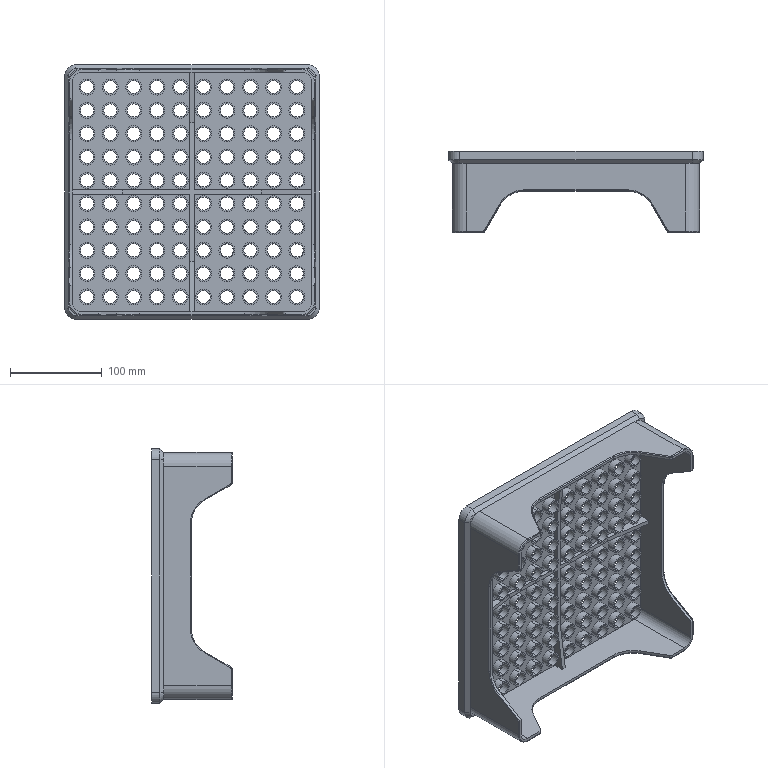Part | 1 solid | 855 faces | box 277 x 88 x 277 mm | volume 456974 mm3 | cylinder 452 | cone 204 | plane 179 | torus 20 | commonest cylinder face diameters 14.2 x200 17.4 x200 2 x20 6 x8 20 x8 60 x8